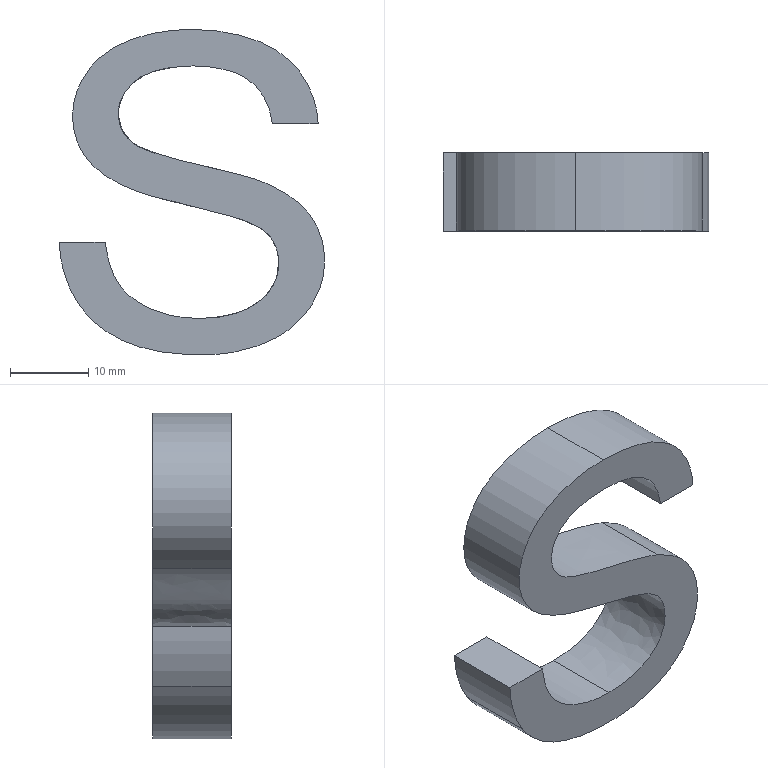Part | NX | features solid 2 | 1 solid | 12 faces | box 33.881 x 10 x 41.56 mm | volume 5827 mm3 | spline 8 | plane 4
STEP:
#1=CARTESIAN_POINT('',(1.866,-915.,225.926));
#2=VERTEX_POINT('',#1);
#3=CARTESIAN_POINT('',(-0.4685,-915.,233.583));
#4=VERTEX_POINT('',#3);
#5=CARTESIAN_POINT('',(1.866,-915.,225.926));
#6=CARTESIAN_POINT('',(0.4034,-915.,228.153));
#7=CARTESIAN_POINT('',(-0.392,-915.,230.723));
#8=CARTESIAN_POINT('',(-0.4685,-915.,233.583));
#9=B_SPLINE_CURVE_WITH_KNOTS('',3,(#5,#6,#7,#8),.UNSPECIFIED.,.F.,.F.,(4,4),(0.,0.03589),.PIECEWISE_BEZIER_KNOTS.);
#10=EDGE_CURVE('',#2,#4,#9,.T.);
#11=ORIENTED_EDGE('',*,*,#10,.F.);
#12=CARTESIAN_POINT('',(1.866,-925.,225.926));
#13=VERTEX_POINT('',#12);
#14=CARTESIAN_POINT('',(1.866,-925.,225.926));
#15=DIRECTION('',(0.,1.,0.));
#16=VECTOR('',#15,1000.);
#17=LINE('',#14,#16);
#18=EDGE_CURVE('',#13,#2,#17,.T.);
#19=ORIENTED_EDGE('',*,*,#18,.F.);
#20=CARTESIAN_POINT('',(-0.4685,-925.,233.583));
#21=VERTEX_POINT('',#20);
#22=CARTESIAN_POINT('',(1.866,-925.,225.926));
#23=CARTESIAN_POINT('',(0.4034,-925.,228.153));
#24=CARTESIAN_POINT('',(-0.392,-925.,230.723));
#25=CARTESIAN_POINT('',(-0.4685,-925.,233.583));
#26=B_SPLINE_CURVE_WITH_KNOTS('',3,(#22,#23,#24,#25),.UNSPECIFIED.,.F.,.F.,(4,4),(0.,0.03589),.PIECEWISE_BEZIER_KNOTS.);
#27=EDGE_CURVE('',#13,#21,#26,.T.);
#28=ORIENTED_EDGE('',*,*,#27,.T.);
#29=CARTESIAN_POINT('',(-0.4685,-925.,233.583));
#30=DIRECTION('',(0.,1.,0.));
#31=VECTOR('',#30,1000.);
#32=LINE('',#29,#31);
#33=EDGE_CURVE('',#21,#4,#32,.T.);
#34=ORIENTED_EDGE('',*,*,#33,.T.);
#35=EDGE_LOOP('',(#11,#19,#28,#34));
#36=FACE_BOUND('',#35,.T.);
#37=CARTESIAN_POINT('',(1.866,-925.,225.926));
#38=CARTESIAN_POINT('',(1.866,-915.,225.926));
#39=CARTESIAN_POINT('',(0.4034,-925.,228.153));
#40=CARTESIAN_POINT('',(0.4034,-915.,228.153));
#41=CARTESIAN_POINT('',(-0.392,-925.,230.723));
#42=CARTESIAN_POINT('',(-0.392,-915.,230.723));
#43=CARTESIAN_POINT('',(-0.4685,-925.,233.583));
#44=CARTESIAN_POINT('',(-0.4685,-915.,233.583));
#45=B_SPLINE_SURFACE_WITH_KNOTS('',3,1,((#37,#38),(#39,#40),(#41,#42),(#43,#44)),.SURF_OF_LINEAR_EXTRUSION.,.F.,.F.,.F.,(4,4),(2,2),(0.,0.03589),(0.,1.),.PIECEWISE_BEZIER_KNOTS.);
#46=ADVANCED_FACE('',(#36),#45,.T.);
#47=CARTESIAN_POINT('',(5.39,-915.,233.583));
#48=VERTEX_POINT('',#47);
#49=CARTESIAN_POINT('',(-0.4685,-915.,233.583));
#50=CARTESIAN_POINT('',(1.484,-915.,233.583));
#51=CARTESIAN_POINT('',(3.437,-915.,233.583));
#52=CARTESIAN_POINT('',(5.39,-915.,233.583));
#53=B_SPLINE_CURVE_WITH_KNOTS('',3,(#49,#50,#51,#52),.UNSPECIFIED.,.F.,.F.,(4,4),(0.03589,0.0618),.PIECEWISE_BEZIER_KNOTS.);
#54=EDGE_CURVE('',#4,#48,#53,.T.);
#55=ORIENTED_EDGE('',*,*,#54,.F.);
#56=ORIENTED_EDGE('',*,*,#33,.F.);
#57=CARTESIAN_POINT('',(5.39,-925.,233.583));
#58=VERTEX_POINT('',#57);
#59=CARTESIAN_POINT('',(-0.4685,-925.,233.583));
#60=CARTESIAN_POINT('',(1.484,-925.,233.583));
#61=CARTESIAN_POINT('',(3.437,-925.,233.583));
#62=CARTESIAN_POINT('',(5.39,-925.,233.583));
#63=B_SPLINE_CURVE_WITH_KNOTS('',3,(#59,#60,#61,#62),.UNSPECIFIED.,.F.,.F.,(4,4),(0.03589,0.0618),.PIECEWISE_BEZIER_KNOTS.);
#64=EDGE_CURVE('',#21,#58,#63,.T.);
#65=ORIENTED_EDGE('',*,*,#64,.T.);
#66=CARTESIAN_POINT('',(5.39,-925.,233.583));
#67=DIRECTION('',(0.,1.,0.));
#68=VECTOR('',#67,1000.);
#69=LINE('',#66,#68);
#70=EDGE_CURVE('',#58,#48,#69,.T.);
#71=ORIENTED_EDGE('',*,*,#70,.T.);
#72=EDGE_LOOP('',(#55,#56,#65,#71));
#73=FACE_BOUND('',#72,.T.);
#74=CARTESIAN_POINT('',(-0.4685,-925.,233.583));
#75=DIRECTION('',(0.,0.,1.));
#76=DIRECTION('',(0.,-1.,0.));
#77=AXIS2_PLACEMENT_3D('',#74,#75,#76);
#78=PLANE('',#77);
#79=ADVANCED_FACE('',(#73),#78,.T.);
#80=CARTESIAN_POINT('',(17.413,-915.,223.885));
#81=VERTEX_POINT('',#80);
#82=CARTESIAN_POINT('',(5.39,-915.,233.583));
#83=CARTESIAN_POINT('',(5.62,-915.,231.457));
#84=CARTESIAN_POINT('',(6.17,-915.,229.698));
#85=CARTESIAN_POINT('',(7.05,-915.,228.362));
#86=CARTESIAN_POINT('',(7.945,-915.,227.006));
#87=CARTESIAN_POINT('',(9.337,-915.,225.935));
#88=CARTESIAN_POINT('',(13.026,-915.,224.275));
#89=CARTESIAN_POINT('',(15.119,-915.,223.855));
#90=CARTESIAN_POINT('',(17.413,-915.,223.885));
#91=B_SPLINE_CURVE_WITH_KNOTS('',3,(#82,#83,#84,#85,#86,#87,#88,#89,#90),.UNSPECIFIED.,.F.,.F.,(4,3,2,4),(0.0618,0.08626,0.1098,0.1336),.UNSPECIFIED.);
#92=EDGE_CURVE('',#48,#81,#91,.T.);
#93=ORIENTED_EDGE('',*,*,#92,.F.);
#94=ORIENTED_EDGE('',*,*,#70,.F.);
#95=CARTESIAN_POINT('',(17.413,-925.,223.885));
#96=VERTEX_POINT('',#95);
#97=CARTESIAN_POINT('',(5.39,-925.,233.583));
#98=CARTESIAN_POINT('',(5.62,-925.,231.457));
#99=CARTESIAN_POINT('',(6.17,-925.,229.698));
#100=CARTESIAN_POINT('',(7.05,-925.,228.362));
#101=CARTESIAN_POINT('',(7.945,-925.,227.006));
#102=CARTESIAN_POINT('',(9.337,-925.,225.935));
#103=CARTESIAN_POINT('',(13.026,-925.,224.275));
#104=CARTESIAN_POINT('',(15.119,-925.,223.855));
#105=CARTESIAN_POINT('',(17.413,-925.,223.885));
#106=B_SPLINE_CURVE_WITH_KNOTS('',3,(#97,#98,#99,#100,#101,#102,#103,#104,#105),.UNSPECIFIED.,.F.,.F.,(4,3,2,4),(0.0618,0.08626,0.1098,0.1336),.UNSPECIFIED.);
#107=EDGE_CURVE('',#58,#96,#106,.T.);
#108=ORIENTED_EDGE('',*,*,#107,.T.);
#109=CARTESIAN_POINT('',(17.413,-925.,223.885));
#110=DIRECTION('',(0.,1.,0.));
#111=VECTOR('',#110,1000.);
#112=LINE('',#109,#111);
#113=EDGE_CURVE('',#96,#81,#112,.T.);
#114=ORIENTED_EDGE('',*,*,#113,.T.);
#115=EDGE_LOOP('',(#93,#94,#108,#114));
#116=FACE_BOUND('',#115,.T.);
#117=CARTESIAN_POINT('',(5.39,-925.,233.583));
#118=CARTESIAN_POINT('',(5.39,-915.,233.583));
#119=CARTESIAN_POINT('',(5.558,-925.,232.023));
#120=CARTESIAN_POINT('',(5.558,-915.,232.023));
#121=CARTESIAN_POINT('',(6.077,-925.,229.978));
#122=CARTESIAN_POINT('',(6.077,-915.,229.978));
#123=CARTESIAN_POINT('',(7.27,-925.,227.917));
#124=CARTESIAN_POINT('',(7.27,-915.,227.917));
#125=CARTESIAN_POINT('',(9.077,-925.,226.092));
#126=CARTESIAN_POINT('',(9.077,-915.,226.092));
#127=CARTESIAN_POINT('',(12.443,-925.,224.339));
#128=CARTESIAN_POINT('',(12.443,-915.,224.339));
#129=CARTESIAN_POINT('',(15.681,-925.,223.862));
#130=CARTESIAN_POINT('',(15.681,-915.,223.862));
#131=CARTESIAN_POINT('',(17.413,-925.,223.885));
#132=CARTESIAN_POINT('',(17.413,-915.,223.885));
#133=B_SPLINE_SURFACE_WITH_KNOTS('',3,1,((#117,#118),(#119,#120),(#121,#122),(#123,#124),(#125,#126),(#127,#128),(#129,#130),(#131,#132)),.SURF_OF_LINEAR_EXTRUSION.,.F.,.F.,.F.,(4,1,1,1,1,4),(2,2),(0.0618,0.07975,0.08872,0.09769,0.1156,0.1336),(0.,1.),.UNSPECIFIED.);
#134=ADVANCED_FACE('',(#116),#133,.T.);
#135=CARTESIAN_POINT('',(7.486,-915.,240.925));
#136=VERTEX_POINT('',#135);
#137=CARTESIAN_POINT('',(17.413,-915.,223.885));
#138=CARTESIAN_POINT('',(19.478,-915.,223.855));
#139=CARTESIAN_POINT('',(21.314,-915.,224.176));
#140=CARTESIAN_POINT('',(24.447,-915.,225.436));
#141=CARTESIAN_POINT('',(25.627,-915.,226.287));
#142=CARTESIAN_POINT('',(26.414,-915.,227.398));
#143=CARTESIAN_POINT('',(27.187,-915.,228.489));
#144=CARTESIAN_POINT('',(27.554,-915.,229.652));
#145=CARTESIAN_POINT('',(27.554,-915.,232.084));
#146=CARTESIAN_POINT('',(27.249,-915.,233.155));
#147=CARTESIAN_POINT('',(26.001,-915.,234.98));
#148=CARTESIAN_POINT('',(24.816,-915.,235.755));
#149=CARTESIAN_POINT('',(23.05,-915.,236.407));
#150=CARTESIAN_POINT('',(21.956,-915.,236.811));
#151=CARTESIAN_POINT('',(19.478,-915.,237.468));
#152=CARTESIAN_POINT('',(11.853,-915.,239.275));
#153=CARTESIAN_POINT('',(9.122,-915.,240.099));
#154=CARTESIAN_POINT('',(7.486,-915.,240.925));
#155=B_SPLINE_CURVE_WITH_KNOTS('',3,(#137,#138,#139,#140,#141,#142,#143,#144,#145,#146,#147,#148,#149,#150,#151,#152,#153,#154),.UNSPECIFIED.,.F.,.F.,(4,2,3,2,2,3,2,4),(0.1336,0.1574,0.1814,0.1978,0.214,0.2299,0.2633,0.2967),.UNSPECIFIED.);
#156=EDGE_CURVE('',#81,#136,#155,.T.);
#157=ORIENTED_EDGE('',*,*,#156,.F.);
#158=ORIENTED_EDGE('',*,*,#113,.F.);
#159=CARTESIAN_POINT('',(7.486,-925.,240.925));
#160=VERTEX_POINT('',#159);
#161=CARTESIAN_POINT('',(17.413,-925.,223.885));
#162=CARTESIAN_POINT('',(19.478,-925.,223.855));
#163=CARTESIAN_POINT('',(21.314,-925.,224.176));
#164=CARTESIAN_POINT('',(24.447,-925.,225.436));
#165=CARTESIAN_POINT('',(25.627,-925.,226.287));
#166=CARTESIAN_POINT('',(26.414,-925.,227.398));
#167=CARTESIAN_POINT('',(27.187,-925.,228.489));
#168=CARTESIAN_POINT('',(27.554,-925.,229.652));
#169=CARTESIAN_POINT('',(27.554,-925.,232.084));
#170=CARTESIAN_POINT('',(27.249,-925.,233.155));
#171=CARTESIAN_POINT('',(26.001,-925.,234.98));
#172=CARTESIAN_POINT('',(24.816,-925.,235.755));
#173=CARTESIAN_POINT('',(23.05,-925.,236.407));
#174=CARTESIAN_POINT('',(21.956,-925.,236.811));
#175=CARTESIAN_POINT('',(19.478,-925.,237.468));
#176=CARTESIAN_POINT('',(11.853,-925.,239.275));
#177=CARTESIAN_POINT('',(9.122,-925.,240.099));
#178=CARTESIAN_POINT('',(7.486,-925.,240.925));
#179=B_SPLINE_CURVE_WITH_KNOTS('',3,(#161,#162,#163,#164,#165,#166,#167,#168,#169,#170,#171,#172,#173,#174,#175,#176,#177,#178),.UNSPECIFIED.,.F.,.F.,(4,2,3,2,2,3,2,4),(0.1336,0.1574,0.1814,0.1978,0.214,0.2299,0.2633,0.2967),.UNSPECIFIED.);
#180=EDGE_CURVE('',#96,#160,#179,.T.);
#181=ORIENTED_EDGE('',*,*,#180,.T.);
#182=CARTESIAN_POINT('',(7.486,-925.,240.925));
#183=DIRECTION('',(0.,1.,0.));
#184=VECTOR('',#183,1000.);
#185=LINE('',#182,#184);
#186=EDGE_CURVE('',#160,#136,#185,.T.);
#187=ORIENTED_EDGE('',*,*,#186,.T.);
#188=EDGE_LOOP('',(#157,#158,#181,#187));
#189=FACE_BOUND('',#188,.T.);
#190=CARTESIAN_POINT('',(17.413,-925.,223.885));
#191=CARTESIAN_POINT('',(17.413,-915.,223.885));
#192=CARTESIAN_POINT('',(19.179,-925.,223.859));
#193=CARTESIAN_POINT('',(19.179,-915.,223.859));
#194=CARTESIAN_POINT('',(21.58,-925.,224.209));
#195=CARTESIAN_POINT('',(21.58,-915.,224.209));
#196=CARTESIAN_POINT('',(24.179,-925.,225.35));
#197=CARTESIAN_POINT('',(24.179,-915.,225.35));
#198=CARTESIAN_POINT('',(25.435,-925.,226.255));
#199=CARTESIAN_POINT('',(25.435,-915.,226.255));
#200=CARTESIAN_POINT('',(26.125,-925.,227.006));
#201=CARTESIAN_POINT('',(26.125,-915.,227.006));
#202=CARTESIAN_POINT('',(26.477,-925.,227.474));
#203=CARTESIAN_POINT('',(26.477,-915.,227.474));
#204=CARTESIAN_POINT('',(26.94,-925.,228.215));
#205=CARTESIAN_POINT('',(26.94,-915.,228.215));
#206=CARTESIAN_POINT('',(27.309,-925.,229.077));
#207=CARTESIAN_POINT('',(27.309,-915.,229.077));
#208=CARTESIAN_POINT('',(27.633,-925.,230.562));
#209=CARTESIAN_POINT('',(27.633,-915.,230.562));
#210=CARTESIAN_POINT('',(27.523,-925.,232.086));
#211=CARTESIAN_POINT('',(27.523,-915.,232.086));
#212=CARTESIAN_POINT('',(27.049,-925.,233.391));
#213=CARTESIAN_POINT('',(27.049,-915.,233.391));
#214=CARTESIAN_POINT('',(26.53,-925.,234.284));
#215=CARTESIAN_POINT('',(26.53,-915.,234.284));
#216=CARTESIAN_POINT('',(25.686,-925.,235.095));
#217=CARTESIAN_POINT('',(25.686,-915.,235.095));
#218=CARTESIAN_POINT('',(24.7,-925.,235.7));
#219=CARTESIAN_POINT('',(24.7,-915.,235.7));
#220=CARTESIAN_POINT('',(23.827,-925.,236.101));
#221=CARTESIAN_POINT('',(23.827,-915.,236.101));
#222=CARTESIAN_POINT('',(23.392,-925.,236.278));
#223=CARTESIAN_POINT('',(23.392,-915.,236.278));
#224=CARTESIAN_POINT('',(23.068,-925.,236.401));
#225=CARTESIAN_POINT('',(23.068,-915.,236.401));
#226=CARTESIAN_POINT('',(22.977,-925.,236.434));
#227=CARTESIAN_POINT('',(22.977,-915.,236.434));
#228=CARTESIAN_POINT('',(22.867,-925.,236.473));
#229=CARTESIAN_POINT('',(22.867,-915.,236.473));
#230=CARTESIAN_POINT('',(22.668,-925.,236.541));
#231=CARTESIAN_POINT('',(22.668,-915.,236.541));
#232=CARTESIAN_POINT('',(22.281,-925.,236.666));
#233=CARTESIAN_POINT('',(22.281,-915.,236.666));
#234=CARTESIAN_POINT('',(21.605,-925.,236.867));
#235=CARTESIAN_POINT('',(21.605,-915.,236.867));
#236=CARTESIAN_POINT('',(20.603,-925.,237.144));
#237=CARTESIAN_POINT('',(20.603,-915.,237.144));
#238=CARTESIAN_POINT('',(19.411,-925.,237.456));
#239=CARTESIAN_POINT('',(19.411,-915.,237.456));
#240=CARTESIAN_POINT('',(18.029,-925.,237.803));
#241=CARTESIAN_POINT('',(18.029,-915.,237.803));
#242=CARTESIAN_POINT('',(16.462,-925.,238.184));
#243=CARTESIAN_POINT('',(16.462,-915.,238.184));
#244=CARTESIAN_POINT('',(14.104,-925.,238.74));
#245=CARTESIAN_POINT('',(14.104,-915.,238.74));
#246=CARTESIAN_POINT('',(11.605,-925.,239.401));
#247=CARTESIAN_POINT('',(11.605,-915.,239.401));
#248=CARTESIAN_POINT('',(9.186,-925.,240.17));
#249=CARTESIAN_POINT('',(9.186,-915.,240.17));
#250=CARTESIAN_POINT('',(7.985,-925.,240.673));
#251=CARTESIAN_POINT('',(7.985,-915.,240.673));
#252=CARTESIAN_POINT('',(7.486,-925.,240.925));
#253=CARTESIAN_POINT('',(7.486,-915.,240.925));
#254=B_SPLINE_SURFACE_WITH_KNOTS('',3,1,((#190,#191),(#192,#193),(#194,#195),(#196,#197),(#198,#199),(#200,#201),(#202,#203),(#204,#205),(#206,#207),(#208,#209),(#210,#211),(#212,#213),(#214,#215),(#216,#217),(#218,#219),(#220,#221),(#222,#223),(#224,#225),(#226,#227),(#228,#229),(#230,#231),(#232,#233),(#234,#235),(#236,#237),(#238,#239),(#240,#241),(#242,#243),(#244,#245),(#246,#247),(#248,#249),(#250,#251),(#252,#253)),.SURF_OF_LINEAR_EXTRUSION.,.F.,.F.,.F.,(4,1,1,1,1,1,1,1,1,1,1,1,1,1,1,1,1,1,1,1,1,1,1,1,1,1,1,1,1,4),(2,2),(0.1336,0.154,0.1642,0.1743,0.1794,0.182,0.1845,0.1896,0.1947,0.2049,0.21,0.2151,0.2202,0.2253,0.2279,0.2291,0.2298,0.2304,0.2317,0.233,0.2355,0.2406,0.2457,0.2508,0.2559,0.261,0.2661,0.2763,0.2865,0.2967),(0.,1.),.UNSPECIFIED.);
#255=ADVANCED_FACE('',(#189),#254,.T.);
#256=CARTESIAN_POINT('',(16.373,-915.,260.78));
#257=VERTEX_POINT('',#256);
#258=CARTESIAN_POINT('',(7.486,-915.,240.925));
#259=CARTESIAN_POINT('',(5.39,-915.,241.889));
#260=CARTESIAN_POINT('',(3.815,-915.,243.128));
#261=CARTESIAN_POINT('',(1.741,-915.,246.116));
#262=CARTESIAN_POINT('',(1.214,-915.,247.793));
#263=CARTESIAN_POINT('',(1.214,-915.,251.679));
#264=CARTESIAN_POINT('',(1.841,-915.,253.56));
#265=CARTESIAN_POINT('',(4.274,-915.,257.088));
#266=CARTESIAN_POINT('',(6.094,-915.,258.44));
#267=CARTESIAN_POINT('',(10.813,-915.,260.309));
#268=CARTESIAN_POINT('',(13.467,-915.,260.75));
#269=CARTESIAN_POINT('',(16.373,-915.,260.78));
#270=B_SPLINE_CURVE_WITH_KNOTS('',3,(#258,#259,#260,#261,#262,#263,#264,#265,#266,#267,#268,#269),.UNSPECIFIED.,.F.,.F.,(4,2,2,2,2,4),(0.2967,0.3228,0.3487,0.3767,0.4045,0.4323),.UNSPECIFIED.);
#271=EDGE_CURVE('',#136,#257,#270,.T.);
#272=ORIENTED_EDGE('',*,*,#271,.F.);
#273=ORIENTED_EDGE('',*,*,#186,.F.);
#274=CARTESIAN_POINT('',(16.373,-925.,260.78));
#275=VERTEX_POINT('',#274);
#276=CARTESIAN_POINT('',(7.486,-925.,240.925));
#277=CARTESIAN_POINT('',(5.39,-925.,241.889));
#278=CARTESIAN_POINT('',(3.815,-925.,243.128));
#279=CARTESIAN_POINT('',(1.741,-925.,246.116));
#280=CARTESIAN_POINT('',(1.214,-925.,247.793));
#281=CARTESIAN_POINT('',(1.214,-925.,251.679));
#282=CARTESIAN_POINT('',(1.841,-925.,253.56));
#283=CARTESIAN_POINT('',(4.274,-925.,257.088));
#284=CARTESIAN_POINT('',(6.094,-925.,258.44));
#285=CARTESIAN_POINT('',(10.813,-925.,260.309));
#286=CARTESIAN_POINT('',(13.467,-925.,260.75));
#287=CARTESIAN_POINT('',(16.373,-925.,260.78));
#288=B_SPLINE_CURVE_WITH_KNOTS('',3,(#276,#277,#278,#279,#280,#281,#282,#283,#284,#285,#286,#287),.UNSPECIFIED.,.F.,.F.,(4,2,2,2,2,4),(0.2967,0.3228,0.3487,0.3767,0.4045,0.4323),.UNSPECIFIED.);
#289=EDGE_CURVE('',#160,#275,#288,.T.);
#290=ORIENTED_EDGE('',*,*,#289,.T.);
#291=CARTESIAN_POINT('',(16.373,-925.,260.78));
#292=DIRECTION('',(0.,1.,0.));
#293=VECTOR('',#292,1000.);
#294=LINE('',#291,#293);
#295=EDGE_CURVE('',#275,#257,#294,.T.);
#296=ORIENTED_EDGE('',*,*,#295,.T.);
#297=EDGE_LOOP('',(#272,#273,#290,#296));
#298=FACE_BOUND('',#297,.T.);
#299=CARTESIAN_POINT('',(7.486,-925.,240.925));
#300=CARTESIAN_POINT('',(7.486,-915.,240.925));
#301=CARTESIAN_POINT('',(4.764,-925.,242.177));
#302=CARTESIAN_POINT('',(4.764,-915.,242.177));
#303=CARTESIAN_POINT('',(2.016,-925.,244.794));
#304=CARTESIAN_POINT('',(2.016,-915.,244.794));
#305=CARTESIAN_POINT('',(1.12,-925.,248.782));
#306=CARTESIAN_POINT('',(1.12,-915.,248.782));
#307=CARTESIAN_POINT('',(1.284,-925.,251.23));
#308=CARTESIAN_POINT('',(1.284,-915.,251.23));
#309=CARTESIAN_POINT('',(1.904,-925.,253.517));
#310=CARTESIAN_POINT('',(1.904,-915.,253.517));
#311=CARTESIAN_POINT('',(3.506,-925.,256.33));
#312=CARTESIAN_POINT('',(3.506,-915.,256.33));
#313=CARTESIAN_POINT('',(6.772,-925.,258.858));
#314=CARTESIAN_POINT('',(6.772,-915.,258.858));
#315=CARTESIAN_POINT('',(11.264,-925.,260.425));
#316=CARTESIAN_POINT('',(11.264,-915.,260.425));
#317=CARTESIAN_POINT('',(14.602,-925.,260.761));
#318=CARTESIAN_POINT('',(14.602,-915.,260.761));
#319=CARTESIAN_POINT('',(16.373,-925.,260.78));
#320=CARTESIAN_POINT('',(16.373,-915.,260.78));
#321=B_SPLINE_SURFACE_WITH_KNOTS('',3,1,((#299,#300),(#301,#302),(#303,#304),(#305,#306),(#307,#308),(#309,#310),(#311,#312),(#313,#314),(#315,#316),(#317,#318),(#319,#320)),.SURF_OF_LINEAR_EXTRUSION.,.F.,.F.,.F.,(4,1,1,1,1,1,1,1,4),(2,2),(0.2967,0.3306,0.3475,0.356,0.3645,0.3814,0.3984,0.4153,0.4323),(0.,1.),.UNSPECIFIED.);
#322=ADVANCED_FACE('',(#298),#321,.T.);
#323=CARTESIAN_POINT('',(32.572,-915.,248.742));
#324=VERTEX_POINT('',#323);
#325=CARTESIAN_POINT('',(16.373,-915.,260.78));
#326=CARTESIAN_POINT('',(19.554,-915.,260.75));
#327=CARTESIAN_POINT('',(22.384,-915.,260.26));
#328=CARTESIAN_POINT('',(27.267,-915.,258.356));
#329=CARTESIAN_POINT('',(29.145,-915.,256.91));
#330=CARTESIAN_POINT('',(30.441,-915.,255.061));
#331=CARTESIAN_POINT('',(31.761,-915.,253.178));
#332=CARTESIAN_POINT('',(32.465,-915.,251.067));
#333=CARTESIAN_POINT('',(32.572,-915.,248.742));
#334=B_SPLINE_CURVE_WITH_KNOTS('',3,(#325,#326,#327,#328,#329,#330,#331,#332,#333),.UNSPECIFIED.,.F.,.F.,(4,2,3,4),(0.4323,0.469,0.5061,0.5353),.UNSPECIFIED.);
#335=EDGE_CURVE('',#257,#324,#334,.T.);
#336=ORIENTED_EDGE('',*,*,#335,.F.);
#337=ORIENTED_EDGE('',*,*,#295,.F.);
#338=CARTESIAN_POINT('',(32.572,-925.,248.742));
#339=VERTEX_POINT('',#338);
#340=CARTESIAN_POINT('',(16.373,-925.,260.78));
#341=CARTESIAN_POINT('',(19.554,-925.,260.75));
#342=CARTESIAN_POINT('',(22.384,-925.,260.26));
#343=CARTESIAN_POINT('',(27.267,-925.,258.356));
#344=CARTESIAN_POINT('',(29.145,-925.,256.91));
#345=CARTESIAN_POINT('',(30.441,-925.,255.061));
#346=CARTESIAN_POINT('',(31.761,-925.,253.178));
#347=CARTESIAN_POINT('',(32.465,-925.,251.067));
#348=CARTESIAN_POINT('',(32.572,-925.,248.742));
#349=B_SPLINE_CURVE_WITH_KNOTS('',3,(#340,#341,#342,#343,#344,#345,#346,#347,#348),.UNSPECIFIED.,.F.,.F.,(4,2,3,4),(0.4323,0.469,0.5061,0.5353),.UNSPECIFIED.);
#350=EDGE_CURVE('',#275,#339,#349,.T.);
#351=ORIENTED_EDGE('',*,*,#350,.T.);
#352=CARTESIAN_POINT('',(32.572,-925.,248.742));
#353=DIRECTION('',(0.,1.,0.));
#354=VECTOR('',#353,1000.);
#355=LINE('',#352,#354);
#356=EDGE_CURVE('',#339,#324,#355,.T.);
#357=ORIENTED_EDGE('',*,*,#356,.T.);
#358=EDGE_LOOP('',(#336,#337,#351,#357));
#359=FACE_BOUND('',#358,.T.);
#360=CARTESIAN_POINT('',(16.373,-925.,260.78));
#361=CARTESIAN_POINT('',(16.373,-915.,260.78));
#362=CARTESIAN_POINT('',(18.602,-925.,260.759));
#363=CARTESIAN_POINT('',(18.602,-915.,260.759));
#364=CARTESIAN_POINT('',(22.71,-925.,260.269));
#365=CARTESIAN_POINT('',(22.71,-915.,260.269));
#366=CARTESIAN_POINT('',(26.929,-925.,258.51));
#367=CARTESIAN_POINT('',(26.929,-915.,258.51));
#368=CARTESIAN_POINT('',(29.094,-925.,256.71));
#369=CARTESIAN_POINT('',(29.094,-915.,256.71));
#370=CARTESIAN_POINT('',(30.015,-925.,255.645));
#371=CARTESIAN_POINT('',(30.015,-915.,255.645));
#372=CARTESIAN_POINT('',(30.458,-925.,255.049));
#373=CARTESIAN_POINT('',(30.458,-915.,255.049));
#374=CARTESIAN_POINT('',(31.045,-925.,254.152));
#375=CARTESIAN_POINT('',(31.045,-915.,254.152));
#376=CARTESIAN_POINT('',(31.597,-925.,253.084));
#377=CARTESIAN_POINT('',(31.597,-915.,253.084));
#378=CARTESIAN_POINT('',(32.283,-925.,251.236));
#379=CARTESIAN_POINT('',(32.283,-915.,251.236));
#380=CARTESIAN_POINT('',(32.525,-925.,249.766));
#381=CARTESIAN_POINT('',(32.525,-915.,249.766));
#382=CARTESIAN_POINT('',(32.572,-925.,248.742));
#383=CARTESIAN_POINT('',(32.572,-915.,248.742));
#384=B_SPLINE_SURFACE_WITH_KNOTS('',3,1,((#360,#361),(#362,#363),(#364,#365),(#366,#367),(#368,#369),(#370,#371),(#372,#373),(#374,#375),(#376,#377),(#378,#379),(#380,#381),(#382,#383)),.SURF_OF_LINEAR_EXTRUSION.,.F.,.F.,.F.,(4,1,1,1,1,1,1,1,1,4),(2,2),(0.4323,0.458,0.4838,0.4967,0.5031,0.5063,0.5096,0.516,0.5224,0.5353),(0.,1.),.UNSPECIFIED.);
#385=ADVANCED_FACE('',(#359),#384,.T.);
#386=CARTESIAN_POINT('',(26.728,-915.,248.742));
#387=VERTEX_POINT('',#386);
#388=CARTESIAN_POINT('',(32.572,-915.,248.742));
#389=CARTESIAN_POINT('',(30.624,-915.,248.742));
#390=CARTESIAN_POINT('',(28.676,-915.,248.742));
#391=CARTESIAN_POINT('',(26.728,-915.,248.742));
#392=B_SPLINE_CURVE_WITH_KNOTS('',3,(#388,#389,#390,#391),.UNSPECIFIED.,.F.,.F.,(4,4),(0.5353,0.5606),.PIECEWISE_BEZIER_KNOTS.);
#393=EDGE_CURVE('',#324,#387,#392,.T.);
#394=ORIENTED_EDGE('',*,*,#393,.F.);
#395=ORIENTED_EDGE('',*,*,#356,.F.);
#396=CARTESIAN_POINT('',(26.728,-925.,248.742));
#397=VERTEX_POINT('',#396);
#398=CARTESIAN_POINT('',(32.572,-925.,248.742));
#399=CARTESIAN_POINT('',(30.624,-925.,248.742));
#400=CARTESIAN_POINT('',(28.676,-925.,248.742));
#401=CARTESIAN_POINT('',(26.728,-925.,248.742));
#402=B_SPLINE_CURVE_WITH_KNOTS('',3,(#398,#399,#400,#401),.UNSPECIFIED.,.F.,.F.,(4,4),(0.5353,0.5606),.PIECEWISE_BEZIER_KNOTS.);
#403=EDGE_CURVE('',#339,#397,#402,.T.);
#404=ORIENTED_EDGE('',*,*,#403,.T.);
#405=CARTESIAN_POINT('',(26.728,-925.,248.742));
#406=DIRECTION('',(0.,1.,0.));
#407=VECTOR('',#406,1000.);
#408=LINE('',#405,#407);
#409=EDGE_CURVE('',#397,#387,#408,.T.);
#410=ORIENTED_EDGE('',*,*,#409,.T.);
#411=EDGE_LOOP('',(#394,#395,#404,#410));
#412=FACE_BOUND('',#411,.T.);
#413=CARTESIAN_POINT('',(32.572,-925.,248.742));
#414=DIRECTION('',(0.,0.,-1.));
#415=DIRECTION('',(0.,1.,0.));
#416=AXIS2_PLACEMENT_3D('',#413,#414,#415);
#417=PLANE('',#416);
#418=ADVANCED_FACE('',(#412),#417,.T.);
#419=CARTESIAN_POINT('',(16.602,-915.,256.115));
#420=VERTEX_POINT('',#419);
#421=CARTESIAN_POINT('',(26.728,-915.,248.742));
#422=CARTESIAN_POINT('',(26.438,-915.,251.143));
#423=CARTESIAN_POINT('',(25.459,-915.,252.964));
#424=CARTESIAN_POINT('',(23.846,-915.,254.209));
#425=CARTESIAN_POINT('',(22.231,-915.,255.457));
#426=CARTESIAN_POINT('',(19.799,-915.,256.084));
#427=CARTESIAN_POINT('',(16.602,-915.,256.115));
#428=B_SPLINE_CURVE_WITH_KNOTS('',3,(#421,#422,#423,#424,#425,#426,#427),.UNSPECIFIED.,.F.,.F.,(4,3,4),(0.5606,0.588,0.621),.PIECEWISE_BEZIER_KNOTS.);
#429=EDGE_CURVE('',#387,#420,#428,.T.);
#430=ORIENTED_EDGE('',*,*,#429,.F.);
#431=ORIENTED_EDGE('',*,*,#409,.F.);
#432=CARTESIAN_POINT('',(16.602,-925.,256.115));
#433=VERTEX_POINT('',#432);
#434=CARTESIAN_POINT('',(26.728,-925.,248.742));
#435=CARTESIAN_POINT('',(26.438,-925.,251.143));
#436=CARTESIAN_POINT('',(25.459,-925.,252.964));
#437=CARTESIAN_POINT('',(23.846,-925.,254.209));
#438=CARTESIAN_POINT('',(22.231,-925.,255.457));
#439=CARTESIAN_POINT('',(19.799,-925.,256.084));
#440=CARTESIAN_POINT('',(16.602,-925.,256.115));
#441=B_SPLINE_CURVE_WITH_KNOTS('',3,(#434,#435,#436,#437,#438,#439,#440),.UNSPECIFIED.,.F.,.F.,(4,3,4),(0.5606,0.588,0.621),.PIECEWISE_BEZIER_KNOTS.);
#442=EDGE_CURVE('',#397,#433,#441,.T.);
#443=ORIENTED_EDGE('',*,*,#442,.T.);
#444=CARTESIAN_POINT('',(16.602,-925.,256.115));
#445=DIRECTION('',(0.,1.,0.));
#446=VECTOR('',#445,1000.);
#447=LINE('',#444,#446);
#448=EDGE_CURVE('',#433,#420,#447,.T.);
#449=ORIENTED_EDGE('',*,*,#448,.T.);
#450=EDGE_LOOP('',(#430,#431,#443,#449));
#451=FACE_BOUND('',#450,.T.);
#452=CARTESIAN_POINT('',(26.728,-925.,248.742));
#453=CARTESIAN_POINT('',(26.728,-915.,248.742));
#454=CARTESIAN_POINT('',(26.569,-925.,250.062));
#455=CARTESIAN_POINT('',(26.569,-915.,250.062));
#456=CARTESIAN_POINT('',(26.008,-925.,251.785));
#457=CARTESIAN_POINT('',(26.008,-915.,251.785));
#458=CARTESIAN_POINT('',(24.863,-925.,253.315));
#459=CARTESIAN_POINT('',(24.863,-915.,253.315));
#460=CARTESIAN_POINT('',(24.019,-925.,254.091));
#461=CARTESIAN_POINT('',(24.019,-915.,254.091));
#462=CARTESIAN_POINT('',(23.242,-925.,254.658));
#463=CARTESIAN_POINT('',(23.242,-915.,254.658));
#464=CARTESIAN_POINT('',(22.141,-925.,255.228));
#465=CARTESIAN_POINT('',(22.141,-915.,255.228));
#466=CARTESIAN_POINT('',(20.025,-925.,255.892));
#467=CARTESIAN_POINT('',(20.025,-915.,255.892));
#468=CARTESIAN_POINT('',(18.068,-925.,256.101));
#469=CARTESIAN_POINT('',(18.068,-915.,256.101));
#470=CARTESIAN_POINT('',(16.602,-925.,256.115));
#471=CARTESIAN_POINT('',(16.602,-915.,256.115));
#472=B_SPLINE_SURFACE_WITH_KNOTS('',3,1,((#452,#453),(#454,#455),(#456,#457),(#458,#459),(#460,#461),(#462,#463),(#464,#465),(#466,#467),(#468,#469),(#470,#471)),.SURF_OF_LINEAR_EXTRUSION.,.F.,.F.,.F.,(4,1,1,1,1,1,1,4),(2,2),(0.5606,0.5757,0.5832,0.587,0.5908,0.5983,0.6059,0.621),(0.,1.),.UNSPECIFIED.);
#473=ADVANCED_FACE('',(#451),#472,.T.);
#474=CARTESIAN_POINT('',(26.193,-915.,241.033));
#475=VERTEX_POINT('',#474);
#476=CARTESIAN_POINT('',(16.602,-915.,256.115));
#477=CARTESIAN_POINT('',(13.283,-915.,256.084));
#478=CARTESIAN_POINT('',(10.851,-915.,255.488));
#479=CARTESIAN_POINT('',(9.351,-915.,254.306));
#480=CARTESIAN_POINT('',(7.822,-915.,253.101));
#481=CARTESIAN_POINT('',(7.057,-915.,251.694));
#482=CARTESIAN_POINT('',(7.057,-915.,248.589));
#483=CARTESIAN_POINT('',(7.608,-915.,247.396));
#484=CARTESIAN_POINT('',(8.652,-915.,246.465));
#485=CARTESIAN_POINT('',(9.734,-915.,245.499));
#486=CARTESIAN_POINT('',(12.503,-915.,244.566));
#487=CARTESIAN_POINT('',(21.439,-915.,242.607));
#488=CARTESIAN_POINT('',(24.526,-915.,241.736));
#489=CARTESIAN_POINT('',(26.193,-915.,241.033));
#490=B_SPLINE_CURVE_WITH_KNOTS('',3,(#476,#477,#478,#479,#480,#481,#482,#483,#484,#485,#486,#487,#488,#489),.UNSPECIFIED.,.F.,.F.,(4,3,2,3,2,4),(0.621,0.6538,0.6756,0.6947,0.7331,0.7715),.UNSPECIFIED.);
#491=EDGE_CURVE('',#420,#475,#490,.T.);
#492=ORIENTED_EDGE('',*,*,#491,.F.);
#493=ORIENTED_EDGE('',*,*,#448,.F.);
#494=CARTESIAN_POINT('',(26.193,-925.,241.033));
#495=VERTEX_POINT('',#494);
#496=CARTESIAN_POINT('',(16.602,-925.,256.115));
#497=CARTESIAN_POINT('',(13.283,-925.,256.084));
#498=CARTESIAN_POINT('',(10.851,-925.,255.488));
#499=CARTESIAN_POINT('',(9.351,-925.,254.306));
#500=CARTESIAN_POINT('',(7.822,-925.,253.101));
#501=CARTESIAN_POINT('',(7.057,-925.,251.694));
#502=CARTESIAN_POINT('',(7.057,-925.,248.589));
#503=CARTESIAN_POINT('',(7.608,-925.,247.396));
#504=CARTESIAN_POINT('',(8.652,-925.,246.465));
#505=CARTESIAN_POINT('',(9.734,-925.,245.499));
#506=CARTESIAN_POINT('',(12.503,-925.,244.566));
#507=CARTESIAN_POINT('',(21.439,-925.,242.607));
#508=CARTESIAN_POINT('',(24.526,-925.,241.736));
#509=CARTESIAN_POINT('',(26.193,-925.,241.033));
#510=B_SPLINE_CURVE_WITH_KNOTS('',3,(#496,#497,#498,#499,#500,#501,#502,#503,#504,#505,#506,#507,#508,#509),.UNSPECIFIED.,.F.,.F.,(4,3,2,3,2,4),(0.621,0.6538,0.6756,0.6947,0.7331,0.7715),.UNSPECIFIED.);
#511=EDGE_CURVE('',#433,#495,#510,.T.);
#512=ORIENTED_EDGE('',*,*,#511,.T.);
#513=CARTESIAN_POINT('',(26.193,-925.,241.033));
#514=DIRECTION('',(0.,1.,0.));
#515=VECTOR('',#514,1000.);
#516=LINE('',#513,#515);
#517=EDGE_CURVE('',#495,#475,#516,.T.);
#518=ORIENTED_EDGE('',*,*,#517,.T.);
#519=EDGE_LOOP('',(#492,#493,#512,#518));
#520=FACE_BOUND('',#519,.T.);
#521=CARTESIAN_POINT('',(16.602,-925.,256.115));
#522=CARTESIAN_POINT('',(16.602,-915.,256.115));
#523=CARTESIAN_POINT('',(14.702,-925.,256.097));
#524=CARTESIAN_POINT('',(14.702,-915.,256.097));
#525=CARTESIAN_POINT('',(12.693,-925.,255.846));
#526=CARTESIAN_POINT('',(12.693,-915.,255.846));
#527=CARTESIAN_POINT('',(10.835,-925.,255.183));
#528=CARTESIAN_POINT('',(10.835,-915.,255.183));
#529=CARTESIAN_POINT('',(10.166,-925.,254.856));
#530=CARTESIAN_POINT('',(10.166,-915.,254.856));
#531=CARTESIAN_POINT('',(9.663,-925.,254.539));
#532=CARTESIAN_POINT('',(9.663,-915.,254.539));
#533=CARTESIAN_POINT('',(9.381,-925.,254.337));
#534=CARTESIAN_POINT('',(9.381,-915.,254.337));
#535=CARTESIAN_POINT('',(8.849,-925.,253.89));
#536=CARTESIAN_POINT('',(8.849,-915.,253.89));
#537=CARTESIAN_POINT('',(8.317,-925.,253.356));
#538=CARTESIAN_POINT('',(8.317,-915.,253.356));
#539=CARTESIAN_POINT('',(7.75,-925.,252.62));
#540=CARTESIAN_POINT('',(7.75,-915.,252.62));
#541=CARTESIAN_POINT('',(7.149,-925.,251.391));
#542=CARTESIAN_POINT('',(7.149,-915.,251.391));
#543=CARTESIAN_POINT('',(6.937,-925.,249.589));
#544=CARTESIAN_POINT('',(6.937,-915.,249.589));
#545=CARTESIAN_POINT('',(7.404,-925.,247.992));
#546=CARTESIAN_POINT('',(7.404,-915.,247.992));
#547=CARTESIAN_POINT('',(8.045,-925.,247.072));
#548=CARTESIAN_POINT('',(8.045,-915.,247.072));
#549=CARTESIAN_POINT('',(8.462,-925.,246.636));
#550=CARTESIAN_POINT('',(8.462,-915.,246.636));
#551=CARTESIAN_POINT('',(8.697,-925.,246.423));
#552=CARTESIAN_POINT('',(8.697,-915.,246.423));
#553=CARTESIAN_POINT('',(8.875,-925.,246.278));
#554=CARTESIAN_POINT('',(8.875,-915.,246.278));
#555=CARTESIAN_POINT('',(9.295,-925.,245.989));
#556=CARTESIAN_POINT('',(9.295,-915.,245.989));
#557=CARTESIAN_POINT('',(10.184,-925.,245.532));
#558=CARTESIAN_POINT('',(10.184,-915.,245.532));
#559=CARTESIAN_POINT('',(11.695,-925.,244.944));
#560=CARTESIAN_POINT('',(11.695,-915.,244.944));
#561=CARTESIAN_POINT('',(13.715,-925.,244.36));
#562=CARTESIAN_POINT('',(13.715,-915.,244.36));
#563=CARTESIAN_POINT('',(15.619,-925.,243.887));
#564=CARTESIAN_POINT('',(15.619,-915.,243.887));
#565=CARTESIAN_POINT('',(17.799,-925.,243.406));
#566=CARTESIAN_POINT('',(17.799,-915.,243.406));
#567=CARTESIAN_POINT('',(20.325,-925.,242.824));
#568=CARTESIAN_POINT('',(20.325,-915.,242.824));
#569=CARTESIAN_POINT('',(23.636,-925.,241.955));
#570=CARTESIAN_POINT('',(23.636,-915.,241.955));
#571=CARTESIAN_POINT('',(25.376,-925.,241.377));
#572=CARTESIAN_POINT('',(25.376,-915.,241.377));
#573=CARTESIAN_POINT('',(26.193,-925.,241.033));
#574=CARTESIAN_POINT('',(26.193,-915.,241.033));
#575=B_SPLINE_SURFACE_WITH_KNOTS('',3,1,((#521,#522),(#523,#524),(#525,#526),(#527,#528),(#529,#530),(#531,#532),(#533,#534),(#535,#536),(#537,#538),(#539,#540),(#541,#542),(#543,#544),(#545,#546),(#547,#548),(#549,#550),(#551,#552),(#553,#554),(#555,#556),(#557,#558),(#559,#560),(#561,#562),(#563,#564),(#565,#566),(#567,#568),(#569,#570),(#571,#572),(#573,#574)),.SURF_OF_LINEAR_EXTRUSION.,.F.,.F.,.F.,(4,1,1,1,1,1,1,1,1,1,1,1,1,1,1,1,1,1,1,1,1,1,1,1,4),(2,2),(0.621,0.6398,0.6445,0.6492,0.6516,0.6539,0.6563,0.6586,0.6633,0.668,0.6774,0.6868,0.6915,0.6939,0.6951,0.6962,0.7009,0.7056,0.7151,0.7245,0.7292,0.7339,0.7433,0.7527,0.7715),(0.,1.),.UNSPECIFIED.);
#576=ADVANCED_FACE('',(#520),#575,.T.);
#577=CARTESIAN_POINT('',(26.193,-915.,241.033));
#578=CARTESIAN_POINT('',(28.656,-915.,239.916));
#579=CARTESIAN_POINT('',(30.491,-915.,238.57));
#580=CARTESIAN_POINT('',(32.822,-915.,235.259));
#581=CARTESIAN_POINT('',(33.413,-915.,233.369));
#582=CARTESIAN_POINT('',(33.413,-915.,229.071));
#583=CARTESIAN_POINT('',(32.786,-915.,227.052));
#584=CARTESIAN_POINT('',(30.173,-915.,223.271));
#585=CARTESIAN_POINT('',(28.319,-915.,221.79));
#586=CARTESIAN_POINT('',(23.45,-915.,219.738));
#587=CARTESIAN_POINT('',(20.702,-915.,219.22));
#588=CARTESIAN_POINT('',(13.834,-915.,219.22));
#589=CARTESIAN_POINT('',(10.621,-915.,219.755));
#590=CARTESIAN_POINT('',(5.39,-915.,221.989));
#591=CARTESIAN_POINT('',(3.356,-915.,223.656));
#592=CARTESIAN_POINT('',(1.866,-915.,225.926));
#593=B_SPLINE_CURVE_WITH_KNOTS('',3,(#577,#578,#579,#580,#581,#582,#583,#584,#585,#586,#587,#588,#589,#590,#591,#592),.UNSPECIFIED.,.F.,.F.,(4,2,2,2,2,2,2,4),(0.7715,0.8013,0.8313,0.8615,0.892,0.9226,0.9613,1.),.UNSPECIFIED.);
#594=EDGE_CURVE('',#475,#2,#593,.T.);
#595=ORIENTED_EDGE('',*,*,#594,.F.);
#596=ORIENTED_EDGE('',*,*,#517,.F.);
#597=CARTESIAN_POINT('',(26.193,-925.,241.033));
#598=CARTESIAN_POINT('',(28.656,-925.,239.916));
#599=CARTESIAN_POINT('',(30.491,-925.,238.57));
#600=CARTESIAN_POINT('',(32.822,-925.,235.259));
#601=CARTESIAN_POINT('',(33.413,-925.,233.369));
#602=CARTESIAN_POINT('',(33.413,-925.,229.071));
#603=CARTESIAN_POINT('',(32.786,-925.,227.052));
#604=CARTESIAN_POINT('',(30.173,-925.,223.271));
#605=CARTESIAN_POINT('',(28.319,-925.,221.79));
#606=CARTESIAN_POINT('',(23.45,-925.,219.738));
#607=CARTESIAN_POINT('',(20.702,-925.,219.22));
#608=CARTESIAN_POINT('',(13.834,-925.,219.22));
#609=CARTESIAN_POINT('',(10.621,-925.,219.755));
#610=CARTESIAN_POINT('',(5.39,-925.,221.989));
#611=CARTESIAN_POINT('',(3.356,-925.,223.656));
#612=CARTESIAN_POINT('',(1.866,-925.,225.926));
#613=B_SPLINE_CURVE_WITH_KNOTS('',3,(#597,#598,#599,#600,#601,#602,#603,#604,#605,#606,#607,#608,#609,#610,#611,#612),.UNSPECIFIED.,.F.,.F.,(4,2,2,2,2,2,2,4),(0.7715,0.8013,0.8313,0.8615,0.892,0.9226,0.9613,1.),.UNSPECIFIED.);
#614=EDGE_CURVE('',#495,#13,#613,.T.);
#615=ORIENTED_EDGE('',*,*,#614,.T.);
#616=ORIENTED_EDGE('',*,*,#18,.T.);
#617=EDGE_LOOP('',(#595,#596,#615,#616));
#618=FACE_BOUND('',#617,.T.);
#619=CARTESIAN_POINT('',(26.193,-925.,241.033));
#620=CARTESIAN_POINT('',(26.193,-915.,241.033));
#621=CARTESIAN_POINT('',(28.549,-925.,239.964));
#622=CARTESIAN_POINT('',(28.549,-915.,239.964));
#623=CARTESIAN_POINT('',(31.205,-925.,238.03));
#624=CARTESIAN_POINT('',(31.205,-915.,238.03));
#625=CARTESIAN_POINT('',(32.974,-925.,234.685));
#626=CARTESIAN_POINT('',(32.974,-915.,234.685));
#627=CARTESIAN_POINT('',(33.535,-925.,231.841));
#628=CARTESIAN_POINT('',(33.535,-915.,231.841));
#629=CARTESIAN_POINT('',(33.28,-925.,228.763));
#630=CARTESIAN_POINT('',(33.28,-915.,228.763));
#631=CARTESIAN_POINT('',(32.152,-925.,225.96));
#632=CARTESIAN_POINT('',(32.152,-915.,225.96));
#633=CARTESIAN_POINT('',(30.143,-925.,223.341));
#634=CARTESIAN_POINT('',(30.143,-915.,223.341));
#635=CARTESIAN_POINT('',(27.444,-925.,221.358));
#636=CARTESIAN_POINT('',(27.444,-915.,221.358));
#637=CARTESIAN_POINT('',(23.956,-925.,219.948));
#638=CARTESIAN_POINT('',(23.956,-915.,219.948));
#639=CARTESIAN_POINT('',(20.147,-925.,219.215));
#640=CARTESIAN_POINT('',(20.147,-915.,219.215));
#641=CARTESIAN_POINT('',(15.831,-925.,219.187));
#642=CARTESIAN_POINT('',(15.831,-915.,219.187));
#643=CARTESIAN_POINT('',(12.061,-925.,219.592));
#644=CARTESIAN_POINT('',(12.061,-915.,219.592));
#645=CARTESIAN_POINT('',(8.779,-925.,220.457));
#646=CARTESIAN_POINT('',(8.779,-915.,220.457));
#647=CARTESIAN_POINT('',(5.059,-925.,222.233));
#648=CARTESIAN_POINT('',(5.059,-915.,222.233));
#649=CARTESIAN_POINT('',(2.965,-925.,224.251));
#650=CARTESIAN_POINT('',(2.965,-915.,224.251));
#651=CARTESIAN_POINT('',(1.866,-925.,225.926));
#652=CARTESIAN_POINT('',(1.866,-915.,225.926));
#653=B_SPLINE_SURFACE_WITH_KNOTS('',3,1,((#619,#620),(#621,#622),(#623,#624),(#625,#626),(#627,#628),(#629,#630),(#631,#632),(#633,#634),(#635,#636),(#637,#638),(#639,#640),(#641,#642),(#643,#644),(#645,#646),(#647,#648),(#649,#650),(#651,#652)),.SURF_OF_LINEAR_EXTRUSION.,.F.,.F.,.F.,(4,1,1,1,1,1,1,1,1,1,1,1,1,1,4),(2,2),(0.7715,0.8001,0.8143,0.8286,0.8429,0.8572,0.8715,0.8857,0.9,0.9143,0.9286,0.9429,0.9572,0.9714,1.),(0.,1.),.UNSPECIFIED.);
#654=ADVANCED_FACE('',(#618),#653,.T.);
#655=ORIENTED_EDGE('',*,*,#27,.F.);
#656=ORIENTED_EDGE('',*,*,#614,.F.);
#657=ORIENTED_EDGE('',*,*,#511,.F.);
#658=ORIENTED_EDGE('',*,*,#442,.F.);
#659=ORIENTED_EDGE('',*,*,#403,.F.);
#660=ORIENTED_EDGE('',*,*,#350,.F.);
#661=ORIENTED_EDGE('',*,*,#289,.F.);
#662=ORIENTED_EDGE('',*,*,#180,.F.);
#663=ORIENTED_EDGE('',*,*,#107,.F.);
#664=ORIENTED_EDGE('',*,*,#64,.F.);
#665=EDGE_LOOP('',(#655,#656,#657,#658,#659,#660,#661,#662,#663,#664));
#666=FACE_BOUND('',#665,.T.);
#667=CARTESIAN_POINT('',(0.1789,-925.,229.517));
#668=DIRECTION('',(0.,-1.,0.));
#669=DIRECTION('',(1.,0.,0.));
#670=AXIS2_PLACEMENT_3D('',#667,#668,#669);
#671=PLANE('',#670);
#672=ADVANCED_FACE('',(#666),#671,.T.);
#673=ORIENTED_EDGE('',*,*,#10,.T.);
#674=ORIENTED_EDGE('',*,*,#54,.T.);
#675=ORIENTED_EDGE('',*,*,#92,.T.);
#676=ORIENTED_EDGE('',*,*,#156,.T.);
#677=ORIENTED_EDGE('',*,*,#271,.T.);
#678=ORIENTED_EDGE('',*,*,#335,.T.);
#679=ORIENTED_EDGE('',*,*,#393,.T.);
#680=ORIENTED_EDGE('',*,*,#429,.T.);
#681=ORIENTED_EDGE('',*,*,#491,.T.);
#682=ORIENTED_EDGE('',*,*,#594,.T.);
#683=EDGE_LOOP('',(#673,#674,#675,#676,#677,#678,#679,#680,#681,#682));
#684=FACE_BOUND('',#683,.T.);
#685=CARTESIAN_POINT('',(0.1789,-915.,229.517));
#686=DIRECTION('',(0.,-1.,0.));
#687=DIRECTION('',(1.,0.,0.));
#688=AXIS2_PLACEMENT_3D('',#685,#686,#687);
#689=PLANE('',#688);
#690=ADVANCED_FACE('',(#684),#689,.F.);
#691=CLOSED_SHELL('',(#46,#79,#134,#255,#322,#385,#418,#473,#576,#654,#672,#690));
#692=MANIFOLD_SOLID_BREP('',#691);
#693=(LENGTH_UNIT()NAMED_UNIT(*)SI_UNIT(.MILLI.,.METRE.));
#694=UNCERTAINTY_MEASURE_WITH_UNIT(LENGTH_MEASURE(0.0508),#693,'','');
#695=(NAMED_UNIT(*)PLANE_ANGLE_UNIT()SI_UNIT($,.RADIAN.));
#696=(NAMED_UNIT(*)SI_UNIT($,.STERADIAN.)SOLID_ANGLE_UNIT());
#697=(GEOMETRIC_REPRESENTATION_CONTEXT(3)GLOBAL_UNCERTAINTY_ASSIGNED_CONTEXT((#694))GLOBAL_UNIT_ASSIGNED_CONTEXT((#693,#695,#696))REPRESENTATION_CONTEXT('',''));
#698=ADVANCED_BREP_SHAPE_REPRESENTATION('',(#692),#697);